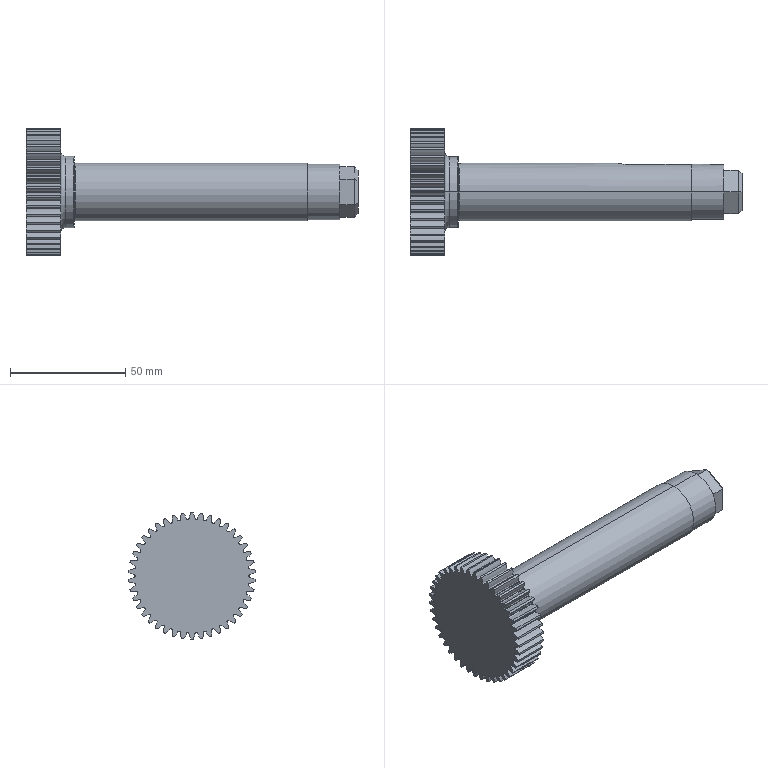Part | SolidWorks | features ICE 7, Chamfer 2, Fillet 2, CirPattern 1, Extrusion 1, RefAxis 1 | 1 solid | 207 faces | box 144 x 54.909 x 55 mm | volume 94342 mm3 | cylinder 94 | spline 84 | plane 23 | torus 4 | cone 2 | commonest cylinder face diameters 55 x43 49.375 x42 24 x2 24.5 x2 25 x2 31 x2